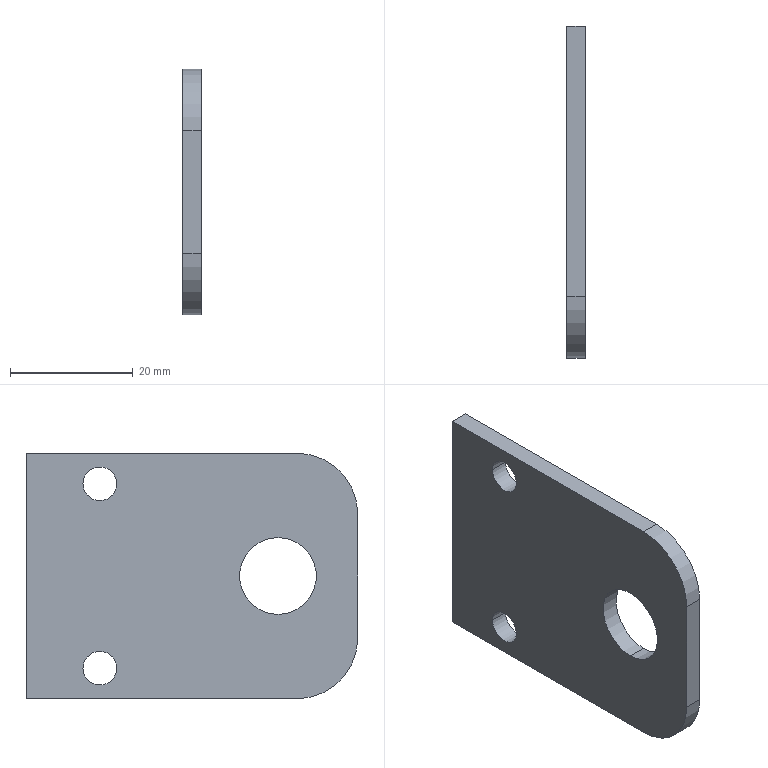Part | STEP file | X77-04023 | 1 solid | 14 faces | box 3 x 54 x 40 mm | volume 5841 mm3 | cylinder 8 | plane 6 | commonest cylinder face diameters 5.5 x4 12.5 x2 20 x2
STEP:
#1=CARTESIAN_POINT('',(0.,-41.,26.25));
#2=VERTEX_POINT('',#1);
#3=CARTESIAN_POINT('',(0.,-41.,13.75));
#4=VERTEX_POINT('',#3);
#5=CARTESIAN_POINT('',(0.,-41.,20.));
#6=DIRECTION('',(1.,0.,0.));
#7=DIRECTION('',(0.,1.,0.));
#8=AXIS2_PLACEMENT_3D('',#5,#6,#7);
#9=CIRCLE('',#8,6.25);
#10=EDGE_CURVE('',#2,#4,#9,.T.);
#11=ORIENTED_EDGE('',*,*,#10,.F.);
#12=CARTESIAN_POINT('',(3.,-41.,26.25));
#13=VERTEX_POINT('',#12);
#14=CARTESIAN_POINT('',(-7.,-41.,26.25));
#15=DIRECTION('',(1.,0.,0.));
#16=VECTOR('',#15,1000.);
#17=LINE('',#14,#16);
#18=EDGE_CURVE('',#2,#13,#17,.T.);
#19=ORIENTED_EDGE('',*,*,#18,.T.);
#20=CARTESIAN_POINT('',(3.,-41.,13.75));
#21=VERTEX_POINT('',#20);
#22=CARTESIAN_POINT('',(3.,-41.,20.));
#23=DIRECTION('',(1.,0.,0.));
#24=DIRECTION('',(0.,0.,-1.));
#25=AXIS2_PLACEMENT_3D('',#22,#23,#24);
#26=CIRCLE('',#25,6.25);
#27=EDGE_CURVE('',#13,#21,#26,.T.);
#28=ORIENTED_EDGE('',*,*,#27,.T.);
#29=CARTESIAN_POINT('',(-7.,-41.,13.75));
#30=DIRECTION('',(1.,0.,0.));
#31=VECTOR('',#30,1000.);
#32=LINE('',#29,#31);
#33=EDGE_CURVE('',#4,#21,#32,.T.);
#34=ORIENTED_EDGE('',*,*,#33,.F.);
#35=EDGE_LOOP('',(#11,#19,#28,#34));
#36=FACE_OUTER_BOUND('',#35,.T.);
#37=CARTESIAN_POINT('',(-7.,-41.,20.));
#38=DIRECTION('',(1.,0.,0.));
#39=DIRECTION('',(0.,0.,-1.));
#40=AXIS2_PLACEMENT_3D('',#37,#38,#39);
#41=CYLINDRICAL_SURFACE('',#40,6.25);
#42=ADVANCED_FACE('',(#36),#41,.F.);
#43=CARTESIAN_POINT('',(3.,-9.25,35.));
#44=VERTEX_POINT('',#43);
#45=CARTESIAN_POINT('',(3.,-14.75,35.));
#46=VERTEX_POINT('',#45);
#47=CARTESIAN_POINT('',(3.,-12.,35.));
#48=DIRECTION('',(-1.,0.,0.));
#49=DIRECTION('',(0.,-1.,0.));
#50=AXIS2_PLACEMENT_3D('',#47,#48,#49);
#51=CIRCLE('',#50,2.75);
#52=EDGE_CURVE('',#44,#46,#51,.T.);
#53=ORIENTED_EDGE('',*,*,#52,.F.);
#54=CARTESIAN_POINT('',(0.,-9.25,35.));
#55=VERTEX_POINT('',#54);
#56=CARTESIAN_POINT('',(3.,-9.25,35.));
#57=DIRECTION('',(-1.,0.,0.));
#58=VECTOR('',#57,1000.);
#59=LINE('',#56,#58);
#60=EDGE_CURVE('',#44,#55,#59,.T.);
#61=ORIENTED_EDGE('',*,*,#60,.T.);
#62=CARTESIAN_POINT('',(0.,-14.75,35.));
#63=VERTEX_POINT('',#62);
#64=CARTESIAN_POINT('',(0.,-12.,35.));
#65=DIRECTION('',(-1.,0.,0.));
#66=DIRECTION('',(0.,-1.,0.));
#67=AXIS2_PLACEMENT_3D('',#64,#65,#66);
#68=CIRCLE('',#67,2.75);
#69=EDGE_CURVE('',#55,#63,#68,.T.);
#70=ORIENTED_EDGE('',*,*,#69,.T.);
#71=CARTESIAN_POINT('',(3.,-14.75,35.));
#72=DIRECTION('',(-1.,0.,0.));
#73=VECTOR('',#72,1000.);
#74=LINE('',#71,#73);
#75=EDGE_CURVE('',#46,#63,#74,.T.);
#76=ORIENTED_EDGE('',*,*,#75,.F.);
#77=EDGE_LOOP('',(#53,#61,#70,#76));
#78=FACE_OUTER_BOUND('',#77,.T.);
#79=CARTESIAN_POINT('',(3.,-12.,35.));
#80=DIRECTION('',(-1.,0.,0.));
#81=DIRECTION('',(0.,-1.,0.));
#82=AXIS2_PLACEMENT_3D('',#79,#80,#81);
#83=CYLINDRICAL_SURFACE('',#82,2.75);
#84=ADVANCED_FACE('',(#78),#83,.F.);
#85=CARTESIAN_POINT('',(3.,-9.25,5.));
#86=VERTEX_POINT('',#85);
#87=CARTESIAN_POINT('',(3.,-14.75,5.));
#88=VERTEX_POINT('',#87);
#89=CARTESIAN_POINT('',(3.,-12.,5.));
#90=DIRECTION('',(-1.,0.,0.));
#91=DIRECTION('',(0.,-1.,0.));
#92=AXIS2_PLACEMENT_3D('',#89,#90,#91);
#93=CIRCLE('',#92,2.75);
#94=EDGE_CURVE('',#86,#88,#93,.T.);
#95=ORIENTED_EDGE('',*,*,#94,.F.);
#96=CARTESIAN_POINT('',(0.,-9.25,5.));
#97=VERTEX_POINT('',#96);
#98=CARTESIAN_POINT('',(3.,-9.25,5.));
#99=DIRECTION('',(-1.,0.,0.));
#100=VECTOR('',#99,1000.);
#101=LINE('',#98,#100);
#102=EDGE_CURVE('',#86,#97,#101,.T.);
#103=ORIENTED_EDGE('',*,*,#102,.T.);
#104=CARTESIAN_POINT('',(0.,-14.75,5.));
#105=VERTEX_POINT('',#104);
#106=CARTESIAN_POINT('',(0.,-12.,5.));
#107=DIRECTION('',(-1.,0.,0.));
#108=DIRECTION('',(0.,-1.,0.));
#109=AXIS2_PLACEMENT_3D('',#106,#107,#108);
#110=CIRCLE('',#109,2.75);
#111=EDGE_CURVE('',#97,#105,#110,.T.);
#112=ORIENTED_EDGE('',*,*,#111,.T.);
#113=CARTESIAN_POINT('',(3.,-14.75,5.));
#114=DIRECTION('',(-1.,0.,0.));
#115=VECTOR('',#114,1000.);
#116=LINE('',#113,#115);
#117=EDGE_CURVE('',#88,#105,#116,.T.);
#118=ORIENTED_EDGE('',*,*,#117,.F.);
#119=EDGE_LOOP('',(#95,#103,#112,#118));
#120=FACE_OUTER_BOUND('',#119,.T.);
#121=CARTESIAN_POINT('',(3.,-12.,5.));
#122=DIRECTION('',(-1.,0.,0.));
#123=DIRECTION('',(0.,-1.,0.));
#124=AXIS2_PLACEMENT_3D('',#121,#122,#123);
#125=CYLINDRICAL_SURFACE('',#124,2.75);
#126=ADVANCED_FACE('',(#120),#125,.F.);
#127=CARTESIAN_POINT('',(3.,0.,0.));
#128=VERTEX_POINT('',#127);
#129=CARTESIAN_POINT('',(0.,0.,0.));
#130=VERTEX_POINT('',#129);
#131=CARTESIAN_POINT('',(3.,0.,0.));
#132=DIRECTION('',(-1.,0.,0.));
#133=VECTOR('',#132,1000.);
#134=LINE('',#131,#133);
#135=EDGE_CURVE('',#128,#130,#134,.T.);
#136=ORIENTED_EDGE('',*,*,#135,.T.);
#137=CARTESIAN_POINT('',(0.,0.,40.));
#138=VERTEX_POINT('',#137);
#139=CARTESIAN_POINT('',(0.,0.,40.));
#140=DIRECTION('',(0.,0.,-1.));
#141=VECTOR('',#140,1000.);
#142=LINE('',#139,#141);
#143=EDGE_CURVE('',#138,#130,#142,.T.);
#144=ORIENTED_EDGE('',*,*,#143,.F.);
#145=CARTESIAN_POINT('',(3.,0.,40.));
#146=VERTEX_POINT('',#145);
#147=CARTESIAN_POINT('',(3.,0.,40.));
#148=DIRECTION('',(-1.,0.,0.));
#149=VECTOR('',#148,1000.);
#150=LINE('',#147,#149);
#151=EDGE_CURVE('',#146,#138,#150,.T.);
#152=ORIENTED_EDGE('',*,*,#151,.F.);
#153=CARTESIAN_POINT('',(3.,0.,40.));
#154=DIRECTION('',(0.,0.,-1.));
#155=VECTOR('',#154,1000.);
#156=LINE('',#153,#155);
#157=EDGE_CURVE('',#146,#128,#156,.T.);
#158=ORIENTED_EDGE('',*,*,#157,.T.);
#159=EDGE_LOOP('',(#136,#144,#152,#158));
#160=FACE_OUTER_BOUND('',#159,.T.);
#161=CARTESIAN_POINT('',(3.,0.,40.));
#162=DIRECTION('',(0.,-1.,0.));
#163=DIRECTION('',(1.,0.,0.));
#164=AXIS2_PLACEMENT_3D('',#161,#162,#163);
#165=PLANE('',#164);
#166=ADVANCED_FACE('',(#160),#165,.F.);
#167=CARTESIAN_POINT('',(0.,-41.,20.));
#168=DIRECTION('',(1.,0.,0.));
#169=DIRECTION('',(0.,1.,0.));
#170=AXIS2_PLACEMENT_3D('',#167,#168,#169);
#171=CIRCLE('',#170,6.25);
#172=EDGE_CURVE('',#4,#2,#171,.T.);
#173=ORIENTED_EDGE('',*,*,#172,.T.);
#174=ORIENTED_EDGE('',*,*,#10,.T.);
#175=EDGE_LOOP('',(#173,#174));
#176=FACE_BOUND('',#175,.T.);
#177=CARTESIAN_POINT('',(0.,-12.,35.));
#178=DIRECTION('',(-1.,0.,0.));
#179=DIRECTION('',(0.,-1.,0.));
#180=AXIS2_PLACEMENT_3D('',#177,#178,#179);
#181=CIRCLE('',#180,2.75);
#182=EDGE_CURVE('',#63,#55,#181,.T.);
#183=ORIENTED_EDGE('',*,*,#182,.F.);
#184=ORIENTED_EDGE('',*,*,#69,.F.);
#185=EDGE_LOOP('',(#183,#184));
#186=FACE_BOUND('',#185,.T.);
#187=CARTESIAN_POINT('',(0.,-12.,5.));
#188=DIRECTION('',(-1.,0.,0.));
#189=DIRECTION('',(0.,-1.,0.));
#190=AXIS2_PLACEMENT_3D('',#187,#188,#189);
#191=CIRCLE('',#190,2.75);
#192=EDGE_CURVE('',#105,#97,#191,.T.);
#193=ORIENTED_EDGE('',*,*,#192,.F.);
#194=ORIENTED_EDGE('',*,*,#111,.F.);
#195=EDGE_LOOP('',(#193,#194));
#196=FACE_BOUND('',#195,.T.);
#197=CARTESIAN_POINT('',(0.,-44.,0.));
#198=VERTEX_POINT('',#197);
#199=CARTESIAN_POINT('',(0.,0.,0.));
#200=DIRECTION('',(0.,-1.,0.));
#201=VECTOR('',#200,1000.);
#202=LINE('',#199,#201);
#203=EDGE_CURVE('',#130,#198,#202,.T.);
#204=ORIENTED_EDGE('',*,*,#203,.T.);
#205=CARTESIAN_POINT('',(0.,-54.,10.));
#206=VERTEX_POINT('',#205);
#207=CARTESIAN_POINT('',(0.,-44.,10.));
#208=DIRECTION('',(-1.,0.,0.));
#209=DIRECTION('',(0.,1.,0.));
#210=AXIS2_PLACEMENT_3D('',#207,#208,#209);
#211=CIRCLE('',#210,10.);
#212=EDGE_CURVE('',#198,#206,#211,.T.);
#213=ORIENTED_EDGE('',*,*,#212,.T.);
#214=CARTESIAN_POINT('',(0.,-54.,30.));
#215=VERTEX_POINT('',#214);
#216=CARTESIAN_POINT('',(0.,-54.,40.));
#217=DIRECTION('',(0.,0.,-1.));
#218=VECTOR('',#217,1000.);
#219=LINE('',#216,#218);
#220=EDGE_CURVE('',#215,#206,#219,.T.);
#221=ORIENTED_EDGE('',*,*,#220,.F.);
#222=CARTESIAN_POINT('',(0.,-44.,40.));
#223=VERTEX_POINT('',#222);
#224=CARTESIAN_POINT('',(0.,-44.,30.));
#225=DIRECTION('',(-1.,0.,0.));
#226=DIRECTION('',(0.,1.,0.));
#227=AXIS2_PLACEMENT_3D('',#224,#225,#226);
#228=CIRCLE('',#227,10.);
#229=EDGE_CURVE('',#215,#223,#228,.T.);
#230=ORIENTED_EDGE('',*,*,#229,.T.);
#231=CARTESIAN_POINT('',(0.,0.,40.));
#232=DIRECTION('',(0.,-1.,0.));
#233=VECTOR('',#232,1000.);
#234=LINE('',#231,#233);
#235=EDGE_CURVE('',#138,#223,#234,.T.);
#236=ORIENTED_EDGE('',*,*,#235,.F.);
#237=ORIENTED_EDGE('',*,*,#143,.T.);
#238=EDGE_LOOP('',(#204,#213,#221,#230,#236,#237));
#239=FACE_OUTER_BOUND('',#238,.T.);
#240=CARTESIAN_POINT('',(0.,0.,40.));
#241=DIRECTION('',(1.,0.,0.));
#242=DIRECTION('',(0.,1.,0.));
#243=AXIS2_PLACEMENT_3D('',#240,#241,#242);
#244=PLANE('',#243);
#245=ADVANCED_FACE('',(#176,#186,#196,#239),#244,.F.);
#246=CARTESIAN_POINT('',(3.,-41.,20.));
#247=DIRECTION('',(1.,0.,0.));
#248=DIRECTION('',(0.,0.,-1.));
#249=AXIS2_PLACEMENT_3D('',#246,#247,#248);
#250=CIRCLE('',#249,6.25);
#251=EDGE_CURVE('',#21,#13,#250,.T.);
#252=ORIENTED_EDGE('',*,*,#251,.F.);
#253=ORIENTED_EDGE('',*,*,#27,.F.);
#254=EDGE_LOOP('',(#252,#253));
#255=FACE_BOUND('',#254,.T.);
#256=CARTESIAN_POINT('',(3.,-12.,35.));
#257=DIRECTION('',(-1.,0.,0.));
#258=DIRECTION('',(0.,-1.,0.));
#259=AXIS2_PLACEMENT_3D('',#256,#257,#258);
#260=CIRCLE('',#259,2.75);
#261=EDGE_CURVE('',#46,#44,#260,.T.);
#262=ORIENTED_EDGE('',*,*,#261,.T.);
#263=ORIENTED_EDGE('',*,*,#52,.T.);
#264=EDGE_LOOP('',(#262,#263));
#265=FACE_BOUND('',#264,.T.);
#266=CARTESIAN_POINT('',(3.,-12.,5.));
#267=DIRECTION('',(-1.,0.,0.));
#268=DIRECTION('',(0.,-1.,0.));
#269=AXIS2_PLACEMENT_3D('',#266,#267,#268);
#270=CIRCLE('',#269,2.75);
#271=EDGE_CURVE('',#88,#86,#270,.T.);
#272=ORIENTED_EDGE('',*,*,#271,.T.);
#273=ORIENTED_EDGE('',*,*,#94,.T.);
#274=EDGE_LOOP('',(#272,#273));
#275=FACE_BOUND('',#274,.T.);
#276=CARTESIAN_POINT('',(3.,-54.,10.));
#277=VERTEX_POINT('',#276);
#278=CARTESIAN_POINT('',(3.,-54.,30.));
#279=VERTEX_POINT('',#278);
#280=CARTESIAN_POINT('',(3.,-54.,40.));
#281=DIRECTION('',(0.,0.,1.));
#282=VECTOR('',#281,1000.);
#283=LINE('',#280,#282);
#284=EDGE_CURVE('',#277,#279,#283,.T.);
#285=ORIENTED_EDGE('',*,*,#284,.F.);
#286=CARTESIAN_POINT('',(3.,-44.,0.));
#287=VERTEX_POINT('',#286);
#288=CARTESIAN_POINT('',(3.,-44.,10.));
#289=DIRECTION('',(1.,0.,0.));
#290=DIRECTION('',(0.,0.,1.));
#291=AXIS2_PLACEMENT_3D('',#288,#289,#290);
#292=CIRCLE('',#291,10.);
#293=EDGE_CURVE('',#277,#287,#292,.T.);
#294=ORIENTED_EDGE('',*,*,#293,.T.);
#295=CARTESIAN_POINT('',(3.,-24.,0.));
#296=DIRECTION('',(0.,1.,0.));
#297=VECTOR('',#296,1000.);
#298=LINE('',#295,#297);
#299=EDGE_CURVE('',#287,#128,#298,.T.);
#300=ORIENTED_EDGE('',*,*,#299,.T.);
#301=ORIENTED_EDGE('',*,*,#157,.F.);
#302=CARTESIAN_POINT('',(3.,-44.,40.));
#303=VERTEX_POINT('',#302);
#304=CARTESIAN_POINT('',(3.,-24.,40.));
#305=DIRECTION('',(0.,1.,0.));
#306=VECTOR('',#305,1000.);
#307=LINE('',#304,#306);
#308=EDGE_CURVE('',#303,#146,#307,.T.);
#309=ORIENTED_EDGE('',*,*,#308,.F.);
#310=CARTESIAN_POINT('',(3.,-44.,30.));
#311=DIRECTION('',(1.,0.,0.));
#312=DIRECTION('',(0.,0.,1.));
#313=AXIS2_PLACEMENT_3D('',#310,#311,#312);
#314=CIRCLE('',#313,10.);
#315=EDGE_CURVE('',#303,#279,#314,.T.);
#316=ORIENTED_EDGE('',*,*,#315,.T.);
#317=EDGE_LOOP('',(#285,#294,#300,#301,#309,#316));
#318=FACE_OUTER_BOUND('',#317,.T.);
#319=CARTESIAN_POINT('',(3.,-24.,40.));
#320=DIRECTION('',(-1.,0.,0.));
#321=DIRECTION('',(0.,0.,1.));
#322=AXIS2_PLACEMENT_3D('',#319,#320,#321);
#323=PLANE('',#322);
#324=ADVANCED_FACE('',(#255,#265,#275,#318),#323,.F.);
#325=ORIENTED_EDGE('',*,*,#235,.T.);
#326=CARTESIAN_POINT('',(0.,-44.,40.));
#327=DIRECTION('',(1.,0.,0.));
#328=VECTOR('',#327,1000.);
#329=LINE('',#326,#328);
#330=EDGE_CURVE('',#223,#303,#329,.T.);
#331=ORIENTED_EDGE('',*,*,#330,.T.);
#332=ORIENTED_EDGE('',*,*,#308,.T.);
#333=ORIENTED_EDGE('',*,*,#151,.T.);
#334=EDGE_LOOP('',(#325,#331,#332,#333));
#335=FACE_OUTER_BOUND('',#334,.T.);
#336=CARTESIAN_POINT('',(0.,0.,40.));
#337=DIRECTION('',(0.,0.,1.));
#338=DIRECTION('',(1.,0.,0.));
#339=AXIS2_PLACEMENT_3D('',#336,#337,#338);
#340=PLANE('',#339);
#341=ADVANCED_FACE('',(#335),#340,.T.);
#342=ORIENTED_EDGE('',*,*,#299,.F.);
#343=CARTESIAN_POINT('',(0.,-44.,0.));
#344=DIRECTION('',(-1.,0.,0.));
#345=VECTOR('',#344,1000.);
#346=LINE('',#343,#345);
#347=EDGE_CURVE('',#287,#198,#346,.T.);
#348=ORIENTED_EDGE('',*,*,#347,.T.);
#349=ORIENTED_EDGE('',*,*,#203,.F.);
#350=ORIENTED_EDGE('',*,*,#135,.F.);
#351=EDGE_LOOP('',(#342,#348,#349,#350));
#352=FACE_OUTER_BOUND('',#351,.T.);
#353=CARTESIAN_POINT('',(0.,0.,0.));
#354=DIRECTION('',(0.,0.,1.));
#355=DIRECTION('',(1.,0.,0.));
#356=AXIS2_PLACEMENT_3D('',#353,#354,#355);
#357=PLANE('',#356);
#358=ADVANCED_FACE('',(#352),#357,.F.);
#359=ORIENTED_EDGE('',*,*,#102,.F.);
#360=ORIENTED_EDGE('',*,*,#271,.F.);
#361=ORIENTED_EDGE('',*,*,#117,.T.);
#362=ORIENTED_EDGE('',*,*,#192,.T.);
#363=EDGE_LOOP('',(#359,#360,#361,#362));
#364=FACE_OUTER_BOUND('',#363,.T.);
#365=CARTESIAN_POINT('',(3.,-12.,5.));
#366=DIRECTION('',(-1.,0.,0.));
#367=DIRECTION('',(0.,-1.,0.));
#368=AXIS2_PLACEMENT_3D('',#365,#366,#367);
#369=CYLINDRICAL_SURFACE('',#368,2.75);
#370=ADVANCED_FACE('',(#364),#369,.F.);
#371=ORIENTED_EDGE('',*,*,#60,.F.);
#372=ORIENTED_EDGE('',*,*,#261,.F.);
#373=ORIENTED_EDGE('',*,*,#75,.T.);
#374=ORIENTED_EDGE('',*,*,#182,.T.);
#375=EDGE_LOOP('',(#371,#372,#373,#374));
#376=FACE_OUTER_BOUND('',#375,.T.);
#377=CARTESIAN_POINT('',(3.,-12.,35.));
#378=DIRECTION('',(-1.,0.,0.));
#379=DIRECTION('',(0.,-1.,0.));
#380=AXIS2_PLACEMENT_3D('',#377,#378,#379);
#381=CYLINDRICAL_SURFACE('',#380,2.75);
#382=ADVANCED_FACE('',(#376),#381,.F.);
#383=ORIENTED_EDGE('',*,*,#220,.T.);
#384=CARTESIAN_POINT('',(3.,-54.,10.));
#385=DIRECTION('',(1.,0.,0.));
#386=VECTOR('',#385,1000.);
#387=LINE('',#384,#386);
#388=EDGE_CURVE('',#206,#277,#387,.T.);
#389=ORIENTED_EDGE('',*,*,#388,.T.);
#390=ORIENTED_EDGE('',*,*,#284,.T.);
#391=CARTESIAN_POINT('',(0.,-54.,30.));
#392=DIRECTION('',(-1.,0.,0.));
#393=VECTOR('',#392,1000.);
#394=LINE('',#391,#393);
#395=EDGE_CURVE('',#279,#215,#394,.T.);
#396=ORIENTED_EDGE('',*,*,#395,.T.);
#397=EDGE_LOOP('',(#383,#389,#390,#396));
#398=FACE_OUTER_BOUND('',#397,.T.);
#399=CARTESIAN_POINT('',(0.,-54.,0.));
#400=DIRECTION('',(0.,-1.,0.));
#401=DIRECTION('',(1.,0.,0.));
#402=AXIS2_PLACEMENT_3D('',#399,#400,#401);
#403=PLANE('',#402);
#404=ADVANCED_FACE('',(#398),#403,.T.);
#405=ORIENTED_EDGE('',*,*,#18,.F.);
#406=ORIENTED_EDGE('',*,*,#172,.F.);
#407=ORIENTED_EDGE('',*,*,#33,.T.);
#408=ORIENTED_EDGE('',*,*,#251,.T.);
#409=EDGE_LOOP('',(#405,#406,#407,#408));
#410=FACE_OUTER_BOUND('',#409,.T.);
#411=CARTESIAN_POINT('',(-7.,-41.,20.));
#412=DIRECTION('',(1.,0.,0.));
#413=DIRECTION('',(0.,0.,-1.));
#414=AXIS2_PLACEMENT_3D('',#411,#412,#413);
#415=CYLINDRICAL_SURFACE('',#414,6.25);
#416=ADVANCED_FACE('',(#410),#415,.F.);
#417=ORIENTED_EDGE('',*,*,#212,.F.);
#418=ORIENTED_EDGE('',*,*,#347,.F.);
#419=ORIENTED_EDGE('',*,*,#293,.F.);
#420=ORIENTED_EDGE('',*,*,#388,.F.);
#421=EDGE_LOOP('',(#417,#418,#419,#420));
#422=FACE_OUTER_BOUND('',#421,.T.);
#423=CARTESIAN_POINT('',(0.,-44.,10.));
#424=DIRECTION('',(-1.,0.,0.));
#425=DIRECTION('',(0.,-1.,0.));
#426=AXIS2_PLACEMENT_3D('',#423,#424,#425);
#427=CYLINDRICAL_SURFACE('',#426,10.);
#428=ADVANCED_FACE('',(#422),#427,.T.);
#429=ORIENTED_EDGE('',*,*,#315,.F.);
#430=ORIENTED_EDGE('',*,*,#330,.F.);
#431=ORIENTED_EDGE('',*,*,#229,.F.);
#432=ORIENTED_EDGE('',*,*,#395,.F.);
#433=EDGE_LOOP('',(#429,#430,#431,#432));
#434=FACE_OUTER_BOUND('',#433,.T.);
#435=CARTESIAN_POINT('',(0.,-44.,30.));
#436=DIRECTION('',(-1.,0.,0.));
#437=DIRECTION('',(0.,-1.,0.));
#438=AXIS2_PLACEMENT_3D('',#435,#436,#437);
#439=CYLINDRICAL_SURFACE('',#438,10.);
#440=ADVANCED_FACE('',(#434),#439,.T.);
#441=CLOSED_SHELL('',(#42,#84,#126,#166,#245,#324,#341,#358,#370,#382,#404,#416,#428,#440));
#442=MANIFOLD_SOLID_BREP('',#441);
#443=CARTESIAN_POINT('',(0.,0.,0.));
#444=DIRECTION('',(0.,0.,1.));
#445=DIRECTION('',(1.,0.,0.));
#446=AXIS2_PLACEMENT_3D('',#443,#444,#445);
#447=(LENGTH_UNIT()NAMED_UNIT(*)SI_UNIT(.MILLI.,.METRE.));
#448=UNCERTAINTY_MEASURE_WITH_UNIT(LENGTH_MEASURE(0.00001),#447,'','');
#449=(NAMED_UNIT(*)PLANE_ANGLE_UNIT()SI_UNIT($,.RADIAN.));
#450=(NAMED_UNIT(*)SI_UNIT($,.STERADIAN.)SOLID_ANGLE_UNIT());
#451=(GEOMETRIC_REPRESENTATION_CONTEXT(3)GLOBAL_UNCERTAINTY_ASSIGNED_CONTEXT((#448))GLOBAL_UNIT_ASSIGNED_CONTEXT((#447,#449,#450))REPRESENTATION_CONTEXT('',''));
#452=ADVANCED_BREP_SHAPE_REPRESENTATION('',(#442,#446),#451);